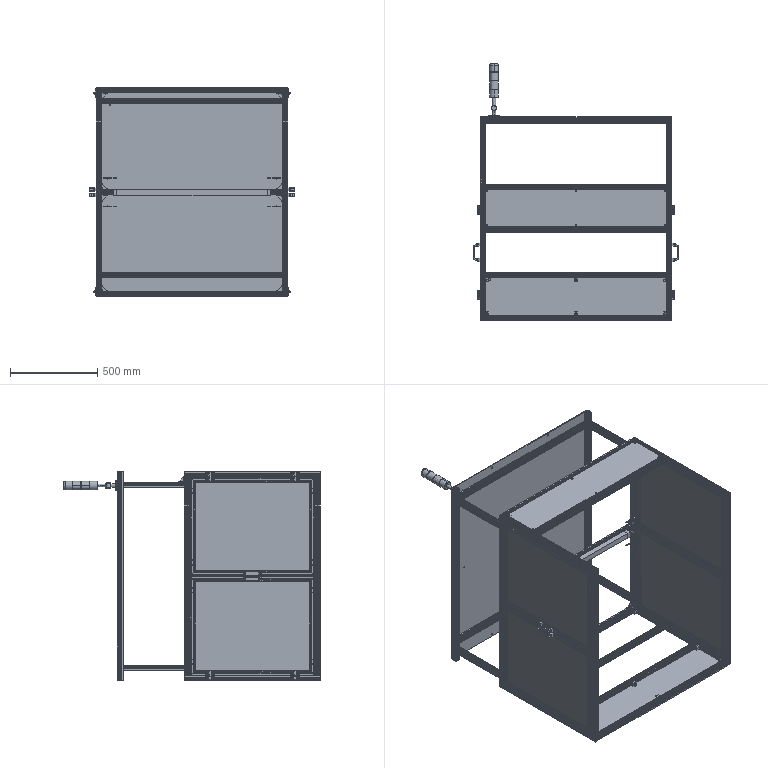Part | SolidWorks | features ReferencePattern 32, MirrorCompFeat 9, InContextFeatHolder 2, LocalLPattern 1 | 147 solids | 7621 faces | volume 31701876 mm3 | plane 4921 | cylinder 1811 | spline 663 | cone 226 | commonest cylinder face diameters 5 x296 6 x184 17.968 x184 14.5 x144 3.3 x128 2 x112